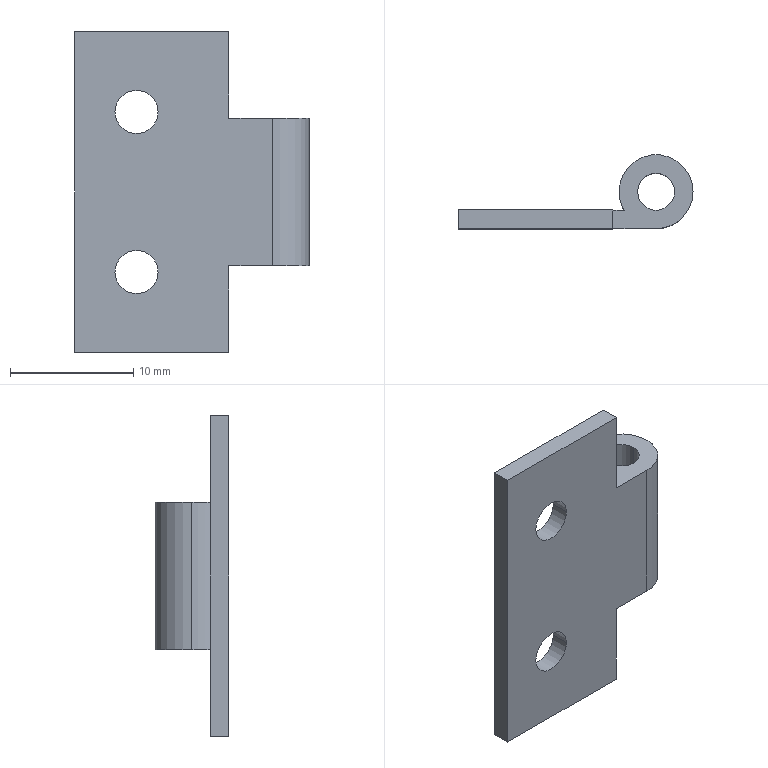Part | SolidWorks | features ICE 3, Extrusion 1 | 1 solid | 18 faces | box 19 x 6 x 26 mm | volume 742.94 mm3 | cylinder 9 | plane 9 | commonest cylinder face diameters 3.5 x4 6 x3 3 x2
STEP:
#1=CARTESIAN_POINT('',(-9.25,-3.,-6.5));
#2=VERTEX_POINT('',#1);
#3=CARTESIAN_POINT('',(-12.75,-3.,-6.5));
#4=VERTEX_POINT('',#3);
#5=CARTESIAN_POINT('',(-11.,-3.,-6.5));
#6=DIRECTION('',(0.,1.,0.));
#7=DIRECTION('',(-1.,0.,0.));
#8=AXIS2_PLACEMENT_3D('',#5,#6,#7);
#9=CIRCLE('',#8,1.75);
#10=EDGE_CURVE('',#2,#4,#9,.T.);
#11=ORIENTED_EDGE('',*,*,#10,.F.);
#12=CARTESIAN_POINT('',(-9.25,-1.5,-6.5));
#13=VERTEX_POINT('',#12);
#14=CARTESIAN_POINT('',(-9.25,-3.,-6.5));
#15=DIRECTION('',(0.,1.,0.));
#16=VECTOR('',#15,1000.);
#17=LINE('',#14,#16);
#18=EDGE_CURVE('',#2,#13,#17,.T.);
#19=ORIENTED_EDGE('',*,*,#18,.T.);
#20=CARTESIAN_POINT('',(-12.75,-1.5,-6.5));
#21=VERTEX_POINT('',#20);
#22=CARTESIAN_POINT('',(-11.,-1.5,-6.5));
#23=DIRECTION('',(0.,1.,0.));
#24=DIRECTION('',(-1.,0.,0.));
#25=AXIS2_PLACEMENT_3D('',#22,#23,#24);
#26=CIRCLE('',#25,1.75);
#27=EDGE_CURVE('',#13,#21,#26,.T.);
#28=ORIENTED_EDGE('',*,*,#27,.T.);
#29=CARTESIAN_POINT('',(-12.75,-3.,-6.5));
#30=DIRECTION('',(0.,1.,0.));
#31=VECTOR('',#30,1000.);
#32=LINE('',#29,#31);
#33=EDGE_CURVE('',#4,#21,#32,.T.);
#34=ORIENTED_EDGE('',*,*,#33,.F.);
#35=EDGE_LOOP('',(#11,#19,#28,#34));
#36=FACE_OUTER_BOUND('',#35,.T.);
#37=CARTESIAN_POINT('',(-11.,-3.,-6.5));
#38=DIRECTION('',(0.,1.,0.));
#39=DIRECTION('',(-1.,0.,0.));
#40=AXIS2_PLACEMENT_3D('',#37,#38,#39);
#41=CYLINDRICAL_SURFACE('',#40,1.75);
#42=ADVANCED_FACE('',(#36),#41,.F.);
#43=CARTESIAN_POINT('',(-9.25,-3.,6.5));
#44=VERTEX_POINT('',#43);
#45=CARTESIAN_POINT('',(-12.75,-3.,6.5));
#46=VERTEX_POINT('',#45);
#47=CARTESIAN_POINT('',(-11.,-3.,6.5));
#48=DIRECTION('',(0.,1.,0.));
#49=DIRECTION('',(1.,0.,0.));
#50=AXIS2_PLACEMENT_3D('',#47,#48,#49);
#51=CIRCLE('',#50,1.75);
#52=EDGE_CURVE('',#44,#46,#51,.T.);
#53=ORIENTED_EDGE('',*,*,#52,.F.);
#54=CARTESIAN_POINT('',(-9.25,-1.5,6.5));
#55=VERTEX_POINT('',#54);
#56=CARTESIAN_POINT('',(-9.25,-3.,6.5));
#57=DIRECTION('',(0.,1.,0.));
#58=VECTOR('',#57,1000.);
#59=LINE('',#56,#58);
#60=EDGE_CURVE('',#44,#55,#59,.T.);
#61=ORIENTED_EDGE('',*,*,#60,.T.);
#62=CARTESIAN_POINT('',(-12.75,-1.5,6.5));
#63=VERTEX_POINT('',#62);
#64=CARTESIAN_POINT('',(-11.,-1.5,6.5));
#65=DIRECTION('',(0.,1.,0.));
#66=DIRECTION('',(1.,0.,0.));
#67=AXIS2_PLACEMENT_3D('',#64,#65,#66);
#68=CIRCLE('',#67,1.75);
#69=EDGE_CURVE('',#55,#63,#68,.T.);
#70=ORIENTED_EDGE('',*,*,#69,.T.);
#71=CARTESIAN_POINT('',(-12.75,-3.,6.5));
#72=DIRECTION('',(0.,1.,0.));
#73=VECTOR('',#72,1000.);
#74=LINE('',#71,#73);
#75=EDGE_CURVE('',#46,#63,#74,.T.);
#76=ORIENTED_EDGE('',*,*,#75,.F.);
#77=EDGE_LOOP('',(#53,#61,#70,#76));
#78=FACE_OUTER_BOUND('',#77,.T.);
#79=CARTESIAN_POINT('',(-11.,-3.,6.5));
#80=DIRECTION('',(0.,1.,0.));
#81=DIRECTION('',(-1.,0.,0.));
#82=AXIS2_PLACEMENT_3D('',#79,#80,#81);
#83=CYLINDRICAL_SURFACE('',#82,1.75);
#84=ADVANCED_FACE('',(#78),#83,.F.);
#85=CARTESIAN_POINT('',(-1.5,0.,6.));
#86=VERTEX_POINT('',#85);
#87=CARTESIAN_POINT('',(1.5,0.,6.));
#88=VERTEX_POINT('',#87);
#89=CARTESIAN_POINT('',(0.,0.,6.));
#90=DIRECTION('',(0.,0.,1.));
#91=DIRECTION('',(1.,0.,0.));
#92=AXIS2_PLACEMENT_3D('',#89,#90,#91);
#93=CIRCLE('',#92,1.5);
#94=EDGE_CURVE('',#86,#88,#93,.T.);
#95=ORIENTED_EDGE('',*,*,#94,.T.);
#96=CARTESIAN_POINT('',(1.5,0.,-6.));
#97=VERTEX_POINT('',#96);
#98=CARTESIAN_POINT('',(1.5,0.,13.));
#99=DIRECTION('',(0.,0.,-1.));
#100=VECTOR('',#99,1000.);
#101=LINE('',#98,#100);
#102=EDGE_CURVE('',#88,#97,#101,.T.);
#103=ORIENTED_EDGE('',*,*,#102,.T.);
#104=CARTESIAN_POINT('',(-1.5,0.,-6.));
#105=VERTEX_POINT('',#104);
#106=CARTESIAN_POINT('',(0.,0.,-6.));
#107=DIRECTION('',(0.,0.,-1.));
#108=DIRECTION('',(-1.,0.,0.));
#109=AXIS2_PLACEMENT_3D('',#106,#107,#108);
#110=CIRCLE('',#109,1.5);
#111=EDGE_CURVE('',#97,#105,#110,.T.);
#112=ORIENTED_EDGE('',*,*,#111,.T.);
#113=CARTESIAN_POINT('',(-1.5,0.,13.));
#114=DIRECTION('',(0.,0.,-1.));
#115=VECTOR('',#114,1000.);
#116=LINE('',#113,#115);
#117=EDGE_CURVE('',#86,#105,#116,.T.);
#118=ORIENTED_EDGE('',*,*,#117,.F.);
#119=EDGE_LOOP('',(#95,#103,#112,#118));
#120=FACE_OUTER_BOUND('',#119,.T.);
#121=CARTESIAN_POINT('',(0.,0.,13.));
#122=DIRECTION('',(0.,0.,-1.));
#123=DIRECTION('',(-1.,0.,0.));
#124=AXIS2_PLACEMENT_3D('',#121,#122,#123);
#125=CYLINDRICAL_SURFACE('',#124,1.5);
#126=ADVANCED_FACE('',(#120),#125,.F.);
#127=CARTESIAN_POINT('',(3.,0.,6.));
#128=VERTEX_POINT('',#127);
#129=CARTESIAN_POINT('',(-3.,0.,6.));
#130=VERTEX_POINT('',#129);
#131=CARTESIAN_POINT('',(0.,0.,6.));
#132=DIRECTION('',(0.,0.,1.));
#133=DIRECTION('',(1.,0.,0.));
#134=AXIS2_PLACEMENT_3D('',#131,#132,#133);
#135=CIRCLE('',#134,3.);
#136=EDGE_CURVE('',#128,#130,#135,.T.);
#137=ORIENTED_EDGE('',*,*,#136,.F.);
#138=CARTESIAN_POINT('',(3.,0.,-6.));
#139=VERTEX_POINT('',#138);
#140=CARTESIAN_POINT('',(3.,0.,13.));
#141=DIRECTION('',(0.,0.,-1.));
#142=VECTOR('',#141,1000.);
#143=LINE('',#140,#142);
#144=EDGE_CURVE('',#128,#139,#143,.T.);
#145=ORIENTED_EDGE('',*,*,#144,.T.);
#146=CARTESIAN_POINT('',(-3.,0.,-6.));
#147=VERTEX_POINT('',#146);
#148=CARTESIAN_POINT('',(0.,0.,-6.));
#149=DIRECTION('',(0.,0.,-1.));
#150=DIRECTION('',(-1.,0.,0.));
#151=AXIS2_PLACEMENT_3D('',#148,#149,#150);
#152=CIRCLE('',#151,3.);
#153=EDGE_CURVE('',#147,#139,#152,.T.);
#154=ORIENTED_EDGE('',*,*,#153,.F.);
#155=CARTESIAN_POINT('',(-3.,0.,13.));
#156=DIRECTION('',(0.,0.,-1.));
#157=VECTOR('',#156,1000.);
#158=LINE('',#155,#157);
#159=EDGE_CURVE('',#130,#147,#158,.T.);
#160=ORIENTED_EDGE('',*,*,#159,.F.);
#161=EDGE_LOOP('',(#137,#145,#154,#160));
#162=FACE_OUTER_BOUND('',#161,.T.);
#163=CARTESIAN_POINT('',(0.,0.,13.));
#164=DIRECTION('',(0.,0.,-1.));
#165=DIRECTION('',(-1.,0.,0.));
#166=AXIS2_PLACEMENT_3D('',#163,#164,#165);
#167=CYLINDRICAL_SURFACE('',#166,3.);
#168=ADVANCED_FACE('',(#162),#167,.T.);
#169=CARTESIAN_POINT('',(-2.598,-1.5,6.));
#170=VERTEX_POINT('',#169);
#171=CARTESIAN_POINT('',(0.,0.,6.));
#172=DIRECTION('',(0.,0.,1.));
#173=DIRECTION('',(1.,0.,0.));
#174=AXIS2_PLACEMENT_3D('',#171,#172,#173);
#175=CIRCLE('',#174,3.);
#176=EDGE_CURVE('',#130,#170,#175,.T.);
#177=ORIENTED_EDGE('',*,*,#176,.F.);
#178=ORIENTED_EDGE('',*,*,#159,.T.);
#179=CARTESIAN_POINT('',(-2.598,-1.5,-6.));
#180=VERTEX_POINT('',#179);
#181=CARTESIAN_POINT('',(0.,0.,-6.));
#182=DIRECTION('',(0.,0.,-1.));
#183=DIRECTION('',(-1.,0.,0.));
#184=AXIS2_PLACEMENT_3D('',#181,#182,#183);
#185=CIRCLE('',#184,3.);
#186=EDGE_CURVE('',#180,#147,#185,.T.);
#187=ORIENTED_EDGE('',*,*,#186,.F.);
#188=CARTESIAN_POINT('',(-2.598,-1.5,13.));
#189=DIRECTION('',(0.,0.,-1.));
#190=VECTOR('',#189,1000.);
#191=LINE('',#188,#190);
#192=EDGE_CURVE('',#170,#180,#191,.T.);
#193=ORIENTED_EDGE('',*,*,#192,.F.);
#194=EDGE_LOOP('',(#177,#178,#187,#193));
#195=FACE_OUTER_BOUND('',#194,.T.);
#196=CARTESIAN_POINT('',(0.,0.,13.));
#197=DIRECTION('',(0.,0.,-1.));
#198=DIRECTION('',(-1.,0.,0.));
#199=AXIS2_PLACEMENT_3D('',#196,#197,#198);
#200=CYLINDRICAL_SURFACE('',#199,3.);
#201=ADVANCED_FACE('',(#195),#200,.T.);
#202=ORIENTED_EDGE('',*,*,#144,.F.);
#203=CARTESIAN_POINT('',(0.,-3.,6.));
#204=VERTEX_POINT('',#203);
#205=CARTESIAN_POINT('',(0.,0.,6.));
#206=DIRECTION('',(0.,0.,1.));
#207=DIRECTION('',(1.,0.,0.));
#208=AXIS2_PLACEMENT_3D('',#205,#206,#207);
#209=CIRCLE('',#208,3.);
#210=EDGE_CURVE('',#204,#128,#209,.T.);
#211=ORIENTED_EDGE('',*,*,#210,.F.);
#212=CARTESIAN_POINT('',(0.,-3.,-6.));
#213=VERTEX_POINT('',#212);
#214=CARTESIAN_POINT('',(0.,-3.,13.));
#215=DIRECTION('',(0.,0.,-1.));
#216=VECTOR('',#215,1000.);
#217=LINE('',#214,#216);
#218=EDGE_CURVE('',#204,#213,#217,.T.);
#219=ORIENTED_EDGE('',*,*,#218,.T.);
#220=CARTESIAN_POINT('',(0.,0.,-6.));
#221=DIRECTION('',(0.,0.,-1.));
#222=DIRECTION('',(-1.,0.,0.));
#223=AXIS2_PLACEMENT_3D('',#220,#221,#222);
#224=CIRCLE('',#223,3.);
#225=EDGE_CURVE('',#139,#213,#224,.T.);
#226=ORIENTED_EDGE('',*,*,#225,.F.);
#227=EDGE_LOOP('',(#202,#211,#219,#226));
#228=FACE_OUTER_BOUND('',#227,.T.);
#229=CARTESIAN_POINT('',(0.,0.,13.));
#230=DIRECTION('',(0.,0.,-1.));
#231=DIRECTION('',(-1.,0.,0.));
#232=AXIS2_PLACEMENT_3D('',#229,#230,#231);
#233=CYLINDRICAL_SURFACE('',#232,3.);
#234=ADVANCED_FACE('',(#228),#233,.T.);
#235=ORIENTED_EDGE('',*,*,#102,.F.);
#236=CARTESIAN_POINT('',(0.,0.,6.));
#237=DIRECTION('',(0.,0.,1.));
#238=DIRECTION('',(1.,0.,0.));
#239=AXIS2_PLACEMENT_3D('',#236,#237,#238);
#240=CIRCLE('',#239,1.5);
#241=EDGE_CURVE('',#88,#86,#240,.T.);
#242=ORIENTED_EDGE('',*,*,#241,.T.);
#243=ORIENTED_EDGE('',*,*,#117,.T.);
#244=CARTESIAN_POINT('',(0.,0.,-6.));
#245=DIRECTION('',(0.,0.,-1.));
#246=DIRECTION('',(-1.,0.,0.));
#247=AXIS2_PLACEMENT_3D('',#244,#245,#246);
#248=CIRCLE('',#247,1.5);
#249=EDGE_CURVE('',#105,#97,#248,.T.);
#250=ORIENTED_EDGE('',*,*,#249,.T.);
#251=EDGE_LOOP('',(#235,#242,#243,#250));
#252=FACE_OUTER_BOUND('',#251,.T.);
#253=CARTESIAN_POINT('',(0.,0.,13.));
#254=DIRECTION('',(0.,0.,-1.));
#255=DIRECTION('',(-1.,0.,0.));
#256=AXIS2_PLACEMENT_3D('',#253,#254,#255);
#257=CYLINDRICAL_SURFACE('',#256,1.5);
#258=ADVANCED_FACE('',(#252),#257,.F.);
#259=CARTESIAN_POINT('',(-3.5,-1.5,13.));
#260=VERTEX_POINT('',#259);
#261=CARTESIAN_POINT('',(-3.5,-3.,13.));
#262=VERTEX_POINT('',#261);
#263=CARTESIAN_POINT('',(-3.5,0.,13.));
#264=DIRECTION('',(0.,-1.,0.));
#265=VECTOR('',#264,1000.);
#266=LINE('',#263,#265);
#267=EDGE_CURVE('',#260,#262,#266,.T.);
#268=ORIENTED_EDGE('',*,*,#267,.F.);
#269=CARTESIAN_POINT('',(-16.,-1.5,13.));
#270=VERTEX_POINT('',#269);
#271=CARTESIAN_POINT('',(-2.598,-1.5,13.));
#272=DIRECTION('',(-1.,0.,0.));
#273=VECTOR('',#272,1000.);
#274=LINE('',#271,#273);
#275=EDGE_CURVE('',#260,#270,#274,.T.);
#276=ORIENTED_EDGE('',*,*,#275,.T.);
#277=CARTESIAN_POINT('',(-16.,-3.,13.));
#278=VERTEX_POINT('',#277);
#279=CARTESIAN_POINT('',(-16.,-1.5,13.));
#280=DIRECTION('',(0.,-1.,0.));
#281=VECTOR('',#280,1000.);
#282=LINE('',#279,#281);
#283=EDGE_CURVE('',#270,#278,#282,.T.);
#284=ORIENTED_EDGE('',*,*,#283,.T.);
#285=CARTESIAN_POINT('',(-16.,-3.,13.));
#286=DIRECTION('',(1.,0.,0.));
#287=VECTOR('',#286,1000.);
#288=LINE('',#285,#287);
#289=EDGE_CURVE('',#278,#262,#288,.T.);
#290=ORIENTED_EDGE('',*,*,#289,.T.);
#291=EDGE_LOOP('',(#268,#276,#284,#290));
#292=FACE_OUTER_BOUND('',#291,.T.);
#293=CARTESIAN_POINT('',(0.,0.,13.));
#294=DIRECTION('',(0.,0.,1.));
#295=DIRECTION('',(1.,0.,0.));
#296=AXIS2_PLACEMENT_3D('',#293,#294,#295);
#297=PLANE('',#296);
#298=ADVANCED_FACE('',(#292),#297,.T.);
#299=CARTESIAN_POINT('',(-3.5,-1.5,-13.));
#300=VERTEX_POINT('',#299);
#301=CARTESIAN_POINT('',(-16.,-1.5,-13.));
#302=VERTEX_POINT('',#301);
#303=CARTESIAN_POINT('',(-2.598,-1.5,-13.));
#304=DIRECTION('',(-1.,0.,0.));
#305=VECTOR('',#304,1000.);
#306=LINE('',#303,#305);
#307=EDGE_CURVE('',#300,#302,#306,.T.);
#308=ORIENTED_EDGE('',*,*,#307,.F.);
#309=CARTESIAN_POINT('',(-3.5,-3.,-13.));
#310=VERTEX_POINT('',#309);
#311=CARTESIAN_POINT('',(-3.5,-3.,-13.));
#312=DIRECTION('',(0.,1.,0.));
#313=VECTOR('',#312,1000.);
#314=LINE('',#311,#313);
#315=EDGE_CURVE('',#310,#300,#314,.T.);
#316=ORIENTED_EDGE('',*,*,#315,.F.);
#317=CARTESIAN_POINT('',(-16.,-3.,-13.));
#318=VERTEX_POINT('',#317);
#319=CARTESIAN_POINT('',(-16.,-3.,-13.));
#320=DIRECTION('',(1.,0.,0.));
#321=VECTOR('',#320,1000.);
#322=LINE('',#319,#321);
#323=EDGE_CURVE('',#318,#310,#322,.T.);
#324=ORIENTED_EDGE('',*,*,#323,.F.);
#325=CARTESIAN_POINT('',(-16.,-1.5,-13.));
#326=DIRECTION('',(0.,-1.,0.));
#327=VECTOR('',#326,1000.);
#328=LINE('',#325,#327);
#329=EDGE_CURVE('',#302,#318,#328,.T.);
#330=ORIENTED_EDGE('',*,*,#329,.F.);
#331=EDGE_LOOP('',(#308,#316,#324,#330));
#332=FACE_OUTER_BOUND('',#331,.T.);
#333=CARTESIAN_POINT('',(0.,0.,-13.));
#334=DIRECTION('',(0.,0.,1.));
#335=DIRECTION('',(1.,0.,0.));
#336=AXIS2_PLACEMENT_3D('',#333,#334,#335);
#337=PLANE('',#336);
#338=ADVANCED_FACE('',(#332),#337,.F.);
#339=ORIENTED_EDGE('',*,*,#329,.T.);
#340=CARTESIAN_POINT('',(-16.,-3.,13.));
#341=DIRECTION('',(0.,0.,-1.));
#342=VECTOR('',#341,1000.);
#343=LINE('',#340,#342);
#344=EDGE_CURVE('',#278,#318,#343,.T.);
#345=ORIENTED_EDGE('',*,*,#344,.F.);
#346=ORIENTED_EDGE('',*,*,#283,.F.);
#347=CARTESIAN_POINT('',(-16.,-1.5,13.));
#348=DIRECTION('',(0.,0.,-1.));
#349=VECTOR('',#348,1000.);
#350=LINE('',#347,#349);
#351=EDGE_CURVE('',#270,#302,#350,.T.);
#352=ORIENTED_EDGE('',*,*,#351,.T.);
#353=EDGE_LOOP('',(#339,#345,#346,#352));
#354=FACE_OUTER_BOUND('',#353,.T.);
#355=CARTESIAN_POINT('',(-16.,-1.5,13.));
#356=DIRECTION('',(1.,0.,0.));
#357=DIRECTION('',(0.,0.,-1.));
#358=AXIS2_PLACEMENT_3D('',#355,#356,#357);
#359=PLANE('',#358);
#360=ADVANCED_FACE('',(#354),#359,.F.);
#361=CARTESIAN_POINT('',(-11.,-3.,-6.5));
#362=DIRECTION('',(0.,1.,0.));
#363=DIRECTION('',(-1.,0.,0.));
#364=AXIS2_PLACEMENT_3D('',#361,#362,#363);
#365=CIRCLE('',#364,1.75);
#366=EDGE_CURVE('',#4,#2,#365,.T.);
#367=ORIENTED_EDGE('',*,*,#366,.T.);
#368=ORIENTED_EDGE('',*,*,#10,.T.);
#369=EDGE_LOOP('',(#367,#368));
#370=FACE_BOUND('',#369,.T.);
#371=CARTESIAN_POINT('',(-11.,-3.,6.5));
#372=DIRECTION('',(0.,1.,0.));
#373=DIRECTION('',(1.,0.,0.));
#374=AXIS2_PLACEMENT_3D('',#371,#372,#373);
#375=CIRCLE('',#374,1.75);
#376=EDGE_CURVE('',#46,#44,#375,.T.);
#377=ORIENTED_EDGE('',*,*,#376,.T.);
#378=ORIENTED_EDGE('',*,*,#52,.T.);
#379=EDGE_LOOP('',(#377,#378));
#380=FACE_BOUND('',#379,.T.);
#381=ORIENTED_EDGE('',*,*,#323,.T.);
#382=CARTESIAN_POINT('',(-3.5,-3.,-6.));
#383=VERTEX_POINT('',#382);
#384=CARTESIAN_POINT('',(-3.5,-3.,-6.));
#385=DIRECTION('',(0.,0.,-1.));
#386=VECTOR('',#385,1000.);
#387=LINE('',#384,#386);
#388=EDGE_CURVE('',#383,#310,#387,.T.);
#389=ORIENTED_EDGE('',*,*,#388,.F.);
#390=CARTESIAN_POINT('',(-1.803,-3.,-6.));
#391=DIRECTION('',(-1.,0.,0.));
#392=VECTOR('',#391,1000.);
#393=LINE('',#390,#392);
#394=EDGE_CURVE('',#213,#383,#393,.T.);
#395=ORIENTED_EDGE('',*,*,#394,.F.);
#396=ORIENTED_EDGE('',*,*,#218,.F.);
#397=CARTESIAN_POINT('',(-3.5,-3.,6.));
#398=VERTEX_POINT('',#397);
#399=CARTESIAN_POINT('',(-3.5,-3.,6.));
#400=DIRECTION('',(1.,0.,0.));
#401=VECTOR('',#400,1000.);
#402=LINE('',#399,#401);
#403=EDGE_CURVE('',#398,#204,#402,.T.);
#404=ORIENTED_EDGE('',*,*,#403,.F.);
#405=CARTESIAN_POINT('',(-3.5,-3.,6.));
#406=DIRECTION('',(0.,0.,1.));
#407=VECTOR('',#406,1000.);
#408=LINE('',#405,#407);
#409=EDGE_CURVE('',#398,#262,#408,.T.);
#410=ORIENTED_EDGE('',*,*,#409,.T.);
#411=ORIENTED_EDGE('',*,*,#289,.F.);
#412=ORIENTED_EDGE('',*,*,#344,.T.);
#413=EDGE_LOOP('',(#381,#389,#395,#396,#404,#410,#411,#412));
#414=FACE_OUTER_BOUND('',#413,.T.);
#415=CARTESIAN_POINT('',(-16.,-3.,13.));
#416=DIRECTION('',(0.,1.,0.));
#417=DIRECTION('',(-1.,0.,0.));
#418=AXIS2_PLACEMENT_3D('',#415,#416,#417);
#419=PLANE('',#418);
#420=ADVANCED_FACE('',(#370,#380,#414),#419,.F.);
#421=CARTESIAN_POINT('',(-11.,-1.5,-6.5));
#422=DIRECTION('',(0.,1.,0.));
#423=DIRECTION('',(-1.,0.,0.));
#424=AXIS2_PLACEMENT_3D('',#421,#422,#423);
#425=CIRCLE('',#424,1.75);
#426=EDGE_CURVE('',#21,#13,#425,.T.);
#427=ORIENTED_EDGE('',*,*,#426,.F.);
#428=ORIENTED_EDGE('',*,*,#27,.F.);
#429=EDGE_LOOP('',(#427,#428));
#430=FACE_BOUND('',#429,.T.);
#431=CARTESIAN_POINT('',(-11.,-1.5,6.5));
#432=DIRECTION('',(0.,1.,0.));
#433=DIRECTION('',(1.,0.,0.));
#434=AXIS2_PLACEMENT_3D('',#431,#432,#433);
#435=CIRCLE('',#434,1.75);
#436=EDGE_CURVE('',#63,#55,#435,.T.);
#437=ORIENTED_EDGE('',*,*,#436,.F.);
#438=ORIENTED_EDGE('',*,*,#69,.F.);
#439=EDGE_LOOP('',(#437,#438));
#440=FACE_BOUND('',#439,.T.);
#441=CARTESIAN_POINT('',(-3.5,-1.5,-6.));
#442=VERTEX_POINT('',#441);
#443=CARTESIAN_POINT('',(-2.598,-1.5,-6.));
#444=DIRECTION('',(1.,0.,0.));
#445=VECTOR('',#444,1000.);
#446=LINE('',#443,#445);
#447=EDGE_CURVE('',#442,#180,#446,.T.);
#448=ORIENTED_EDGE('',*,*,#447,.F.);
#449=CARTESIAN_POINT('',(-3.5,-1.5,13.));
#450=DIRECTION('',(0.,0.,-1.));
#451=VECTOR('',#450,1000.);
#452=LINE('',#449,#451);
#453=EDGE_CURVE('',#442,#300,#452,.T.);
#454=ORIENTED_EDGE('',*,*,#453,.T.);
#455=ORIENTED_EDGE('',*,*,#307,.T.);
#456=ORIENTED_EDGE('',*,*,#351,.F.);
#457=ORIENTED_EDGE('',*,*,#275,.F.);
#458=CARTESIAN_POINT('',(-3.5,-1.5,6.));
#459=VERTEX_POINT('',#458);
#460=CARTESIAN_POINT('',(-3.5,-1.5,13.));
#461=DIRECTION('',(0.,0.,-1.));
#462=VECTOR('',#461,1000.);
#463=LINE('',#460,#462);
#464=EDGE_CURVE('',#260,#459,#463,.T.);
#465=ORIENTED_EDGE('',*,*,#464,.T.);
#466=CARTESIAN_POINT('',(-2.598,-1.5,6.));
#467=DIRECTION('',(-1.,0.,0.));
#468=VECTOR('',#467,1000.);
#469=LINE('',#466,#468);
#470=EDGE_CURVE('',#170,#459,#469,.T.);
#471=ORIENTED_EDGE('',*,*,#470,.F.);
#472=ORIENTED_EDGE('',*,*,#192,.T.);
#473=EDGE_LOOP('',(#448,#454,#455,#456,#457,#465,#471,#472));
#474=FACE_OUTER_BOUND('',#473,.T.);
#475=CARTESIAN_POINT('',(-2.598,-1.5,13.));
#476=DIRECTION('',(0.,-1.,0.));
#477=DIRECTION('',(1.,0.,0.));
#478=AXIS2_PLACEMENT_3D('',#475,#476,#477);
#479=PLANE('',#478);
#480=ADVANCED_FACE('',(#430,#440,#474),#479,.F.);
#481=ORIENTED_EDGE('',*,*,#267,.T.);
#482=ORIENTED_EDGE('',*,*,#409,.F.);
#483=CARTESIAN_POINT('',(-3.5,0.,6.));
#484=DIRECTION('',(0.,-1.,0.));
#485=VECTOR('',#484,1000.);
#486=LINE('',#483,#485);
#487=EDGE_CURVE('',#459,#398,#486,.T.);
#488=ORIENTED_EDGE('',*,*,#487,.F.);
#489=ORIENTED_EDGE('',*,*,#464,.F.);
#490=EDGE_LOOP('',(#481,#482,#488,#489));
#491=FACE_OUTER_BOUND('',#490,.T.);
#492=CARTESIAN_POINT('',(-3.5,0.,6.));
#493=DIRECTION('',(-1.,0.,0.));
#494=DIRECTION('',(0.,-1.,0.));
#495=AXIS2_PLACEMENT_3D('',#492,#493,#494);
#496=PLANE('',#495);
#497=ADVANCED_FACE('',(#491),#496,.F.);
#498=ORIENTED_EDGE('',*,*,#94,.F.);
#499=ORIENTED_EDGE('',*,*,#241,.F.);
#500=EDGE_LOOP('',(#498,#499));
#501=FACE_BOUND('',#500,.T.);
#502=ORIENTED_EDGE('',*,*,#403,.T.);
#503=ORIENTED_EDGE('',*,*,#210,.T.);
#504=ORIENTED_EDGE('',*,*,#136,.T.);
#505=ORIENTED_EDGE('',*,*,#176,.T.);
#506=ORIENTED_EDGE('',*,*,#470,.T.);
#507=ORIENTED_EDGE('',*,*,#487,.T.);
#508=EDGE_LOOP('',(#502,#503,#504,#505,#506,#507));
#509=FACE_OUTER_BOUND('',#508,.T.);
#510=CARTESIAN_POINT('',(0.,0.,6.));
#511=DIRECTION('',(0.,0.,1.));
#512=DIRECTION('',(1.,0.,0.));
#513=AXIS2_PLACEMENT_3D('',#510,#511,#512);
#514=PLANE('',#513);
#515=ADVANCED_FACE('',(#501,#509),#514,.T.);
#516=CARTESIAN_POINT('',(-3.5,-3.,-6.));
#517=DIRECTION('',(0.,1.,0.));
#518=VECTOR('',#517,1000.);
#519=LINE('',#516,#518);
#520=EDGE_CURVE('',#383,#442,#519,.T.);
#521=ORIENTED_EDGE('',*,*,#520,.F.);
#522=ORIENTED_EDGE('',*,*,#388,.T.);
#523=ORIENTED_EDGE('',*,*,#315,.T.);
#524=ORIENTED_EDGE('',*,*,#453,.F.);
#525=EDGE_LOOP('',(#521,#522,#523,#524));
#526=FACE_OUTER_BOUND('',#525,.T.);
#527=CARTESIAN_POINT('',(-3.5,-3.,-6.));
#528=DIRECTION('',(-1.,0.,0.));
#529=DIRECTION('',(0.,-1.,0.));
#530=AXIS2_PLACEMENT_3D('',#527,#528,#529);
#531=PLANE('',#530);
#532=ADVANCED_FACE('',(#526),#531,.F.);
#533=ORIENTED_EDGE('',*,*,#249,.F.);
#534=ORIENTED_EDGE('',*,*,#111,.F.);
#535=EDGE_LOOP('',(#533,#534));
#536=FACE_BOUND('',#535,.T.);
#537=ORIENTED_EDGE('',*,*,#186,.T.);
#538=ORIENTED_EDGE('',*,*,#153,.T.);
#539=ORIENTED_EDGE('',*,*,#225,.T.);
#540=ORIENTED_EDGE('',*,*,#394,.T.);
#541=ORIENTED_EDGE('',*,*,#520,.T.);
#542=ORIENTED_EDGE('',*,*,#447,.T.);
#543=EDGE_LOOP('',(#537,#538,#539,#540,#541,#542));
#544=FACE_OUTER_BOUND('',#543,.T.);
#545=CARTESIAN_POINT('',(0.,0.,-6.));
#546=DIRECTION('',(0.,0.,-1.));
#547=DIRECTION('',(-1.,0.,0.));
#548=AXIS2_PLACEMENT_3D('',#545,#546,#547);
#549=PLANE('',#548);
#550=ADVANCED_FACE('',(#536,#544),#549,.T.);
#551=ORIENTED_EDGE('',*,*,#60,.F.);
#552=ORIENTED_EDGE('',*,*,#376,.F.);
#553=ORIENTED_EDGE('',*,*,#75,.T.);
#554=ORIENTED_EDGE('',*,*,#436,.T.);
#555=EDGE_LOOP('',(#551,#552,#553,#554));
#556=FACE_OUTER_BOUND('',#555,.T.);
#557=CARTESIAN_POINT('',(-11.,-3.,6.5));
#558=DIRECTION('',(0.,1.,0.));
#559=DIRECTION('',(-1.,0.,0.));
#560=AXIS2_PLACEMENT_3D('',#557,#558,#559);
#561=CYLINDRICAL_SURFACE('',#560,1.75);
#562=ADVANCED_FACE('',(#556),#561,.F.);
#563=ORIENTED_EDGE('',*,*,#18,.F.);
#564=ORIENTED_EDGE('',*,*,#366,.F.);
#565=ORIENTED_EDGE('',*,*,#33,.T.);
#566=ORIENTED_EDGE('',*,*,#426,.T.);
#567=EDGE_LOOP('',(#563,#564,#565,#566));
#568=FACE_OUTER_BOUND('',#567,.T.);
#569=CARTESIAN_POINT('',(-11.,-3.,-6.5));
#570=DIRECTION('',(0.,1.,0.));
#571=DIRECTION('',(-1.,0.,0.));
#572=AXIS2_PLACEMENT_3D('',#569,#570,#571);
#573=CYLINDRICAL_SURFACE('',#572,1.75);
#574=ADVANCED_FACE('',(#568),#573,.F.);
#575=CLOSED_SHELL('',(#42,#84,#126,#168,#201,#234,#258,#298,#338,#360,#420,#480,#497,#515,#532,#550,#562,#574));
#576=MANIFOLD_SOLID_BREP('',#575);
#577=CARTESIAN_POINT('',(0.,0.,0.));
#578=DIRECTION('',(0.,0.,1.));
#579=DIRECTION('',(1.,0.,0.));
#580=AXIS2_PLACEMENT_3D('',#577,#578,#579);
#581=(LENGTH_UNIT()NAMED_UNIT(*)SI_UNIT(.MILLI.,.METRE.));
#582=UNCERTAINTY_MEASURE_WITH_UNIT(LENGTH_MEASURE(0.00001),#581,'','');
#583=(NAMED_UNIT(*)PLANE_ANGLE_UNIT()SI_UNIT($,.RADIAN.));
#584=(NAMED_UNIT(*)SI_UNIT($,.STERADIAN.)SOLID_ANGLE_UNIT());
#585=(GEOMETRIC_REPRESENTATION_CONTEXT(3)GLOBAL_UNCERTAINTY_ASSIGNED_CONTEXT((#582))GLOBAL_UNIT_ASSIGNED_CONTEXT((#581,#583,#584))REPRESENTATION_CONTEXT('',''));
#586=ADVANCED_BREP_SHAPE_REPRESENTATION('',(#576,#580),#585);